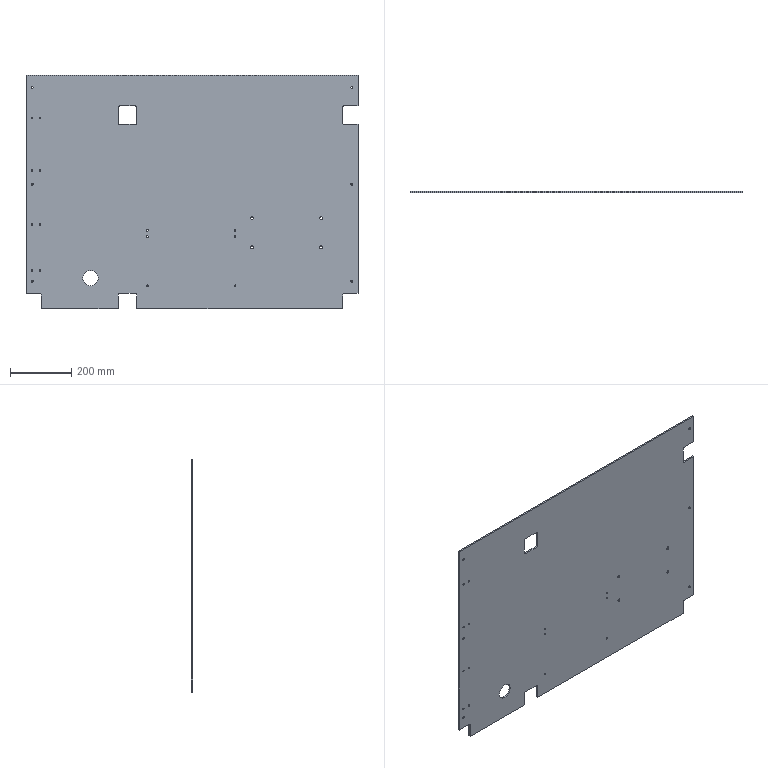Part | SolidWorks | features BaseBody 1 | 1 solid | 94 faces | box 1080 x 5 x 760 mm | volume 4016993 mm3 | cylinder 60 | plane 22 | cone 12 | commonest cylinder face diameters 5 x28 6.6 x12 10 x10 9 x8 50 x2